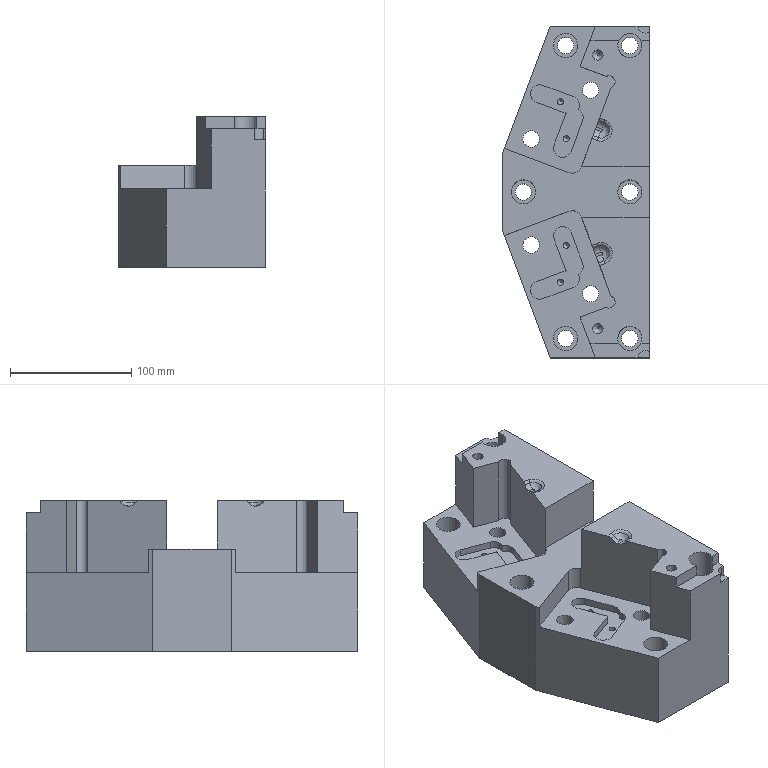Part | NX | features 23 2 | 1 solid | 116 faces | box 121 x 274 x 124.5 mm | volume 2383113 mm3 | plane 56 | cylinder 50 | cone 6 | spline 4 | commonest cylinder face diameters 13.5 x10 15 x10 20 x10 5.2 x4 6 x4 13 x4